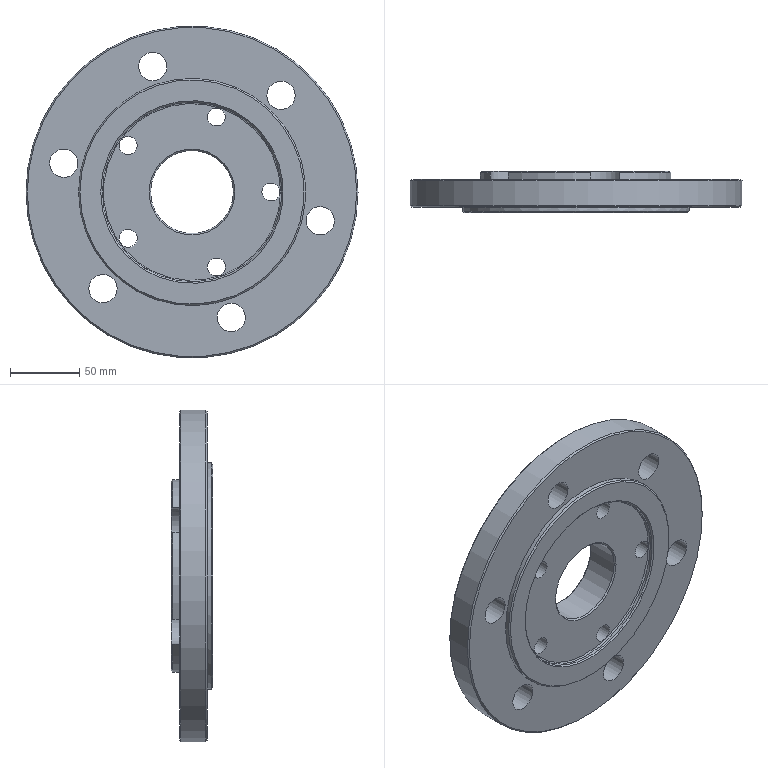Part | STEP file | HL4GZ-1.313.204 (front wheel mounting plate) | 1 solid | 47 faces | box 240 x 30.001 x 240 mm | volume 849969 mm3 | cylinder 25 | cone 11 | plane 10 | torus 1 | commonest cylinder face diameters 20.5 x6 13 x5 32 x5 139 x5 60 x1 130 x1